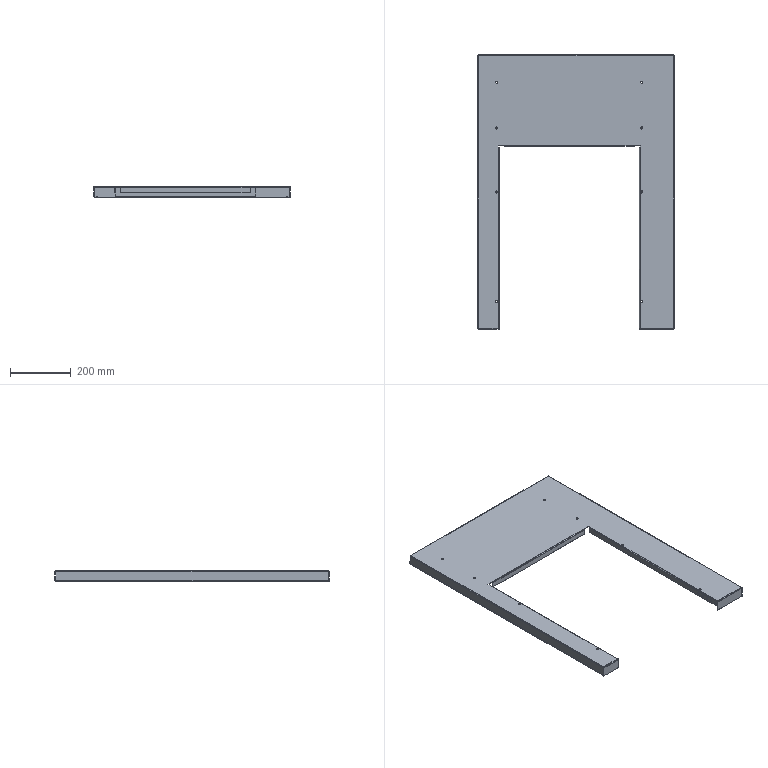Part | SolidWorks | features ICE 6, EdgeFlange 5, FlatPattern 1, SMBaseFlange 1, SheetMetal 1 | 1 solid | 140 faces | box 645 x 900 x 35 mm | volume 874685 mm3 | plane 70 | cylinder 58 | spline 12 | commonest cylinder face diameters 6.8 x20 7 x16 2 x11 6 x11